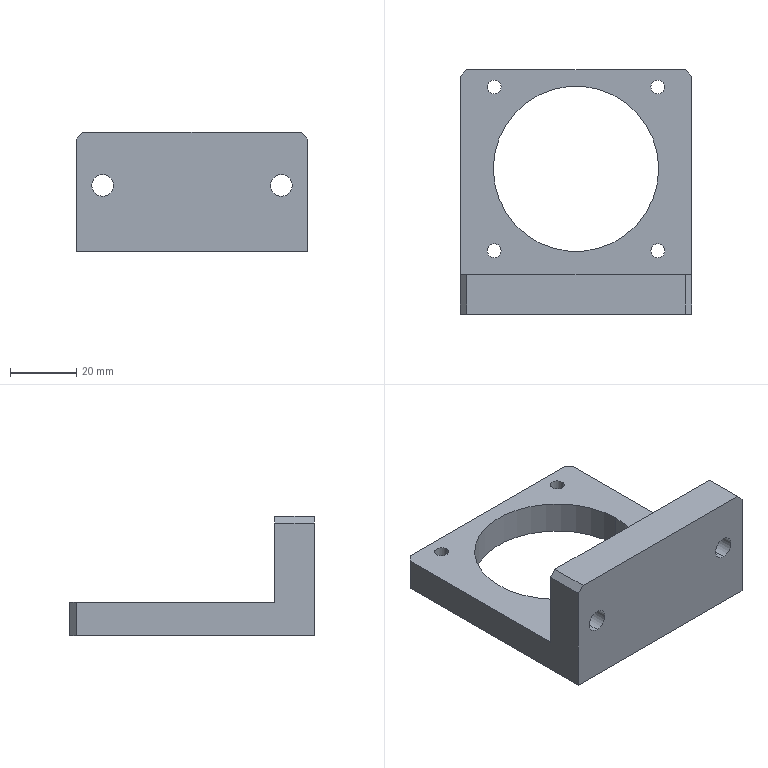Part | NX | features BREP 1 | 1 solid | 32 faces | box 70 x 74 x 36 mm | volume 51715 mm3 | cylinder 18 | plane 14 | commonest cylinder face diameters 4.2 x8 6.6 x4 11 x4 50 x2
STEP:
#1=CARTESIAN_POINT('',(33.,74.,0.));
#2=VERTEX_POINT('',#1);
#3=CARTESIAN_POINT('',(35.,72.,0.));
#4=VERTEX_POINT('',#3);
#5=CARTESIAN_POINT('',(35.,72.,0.));
#6=DIRECTION('',(0.7071,-0.7071,0.));
#7=VECTOR('',#6,1000.);
#8=LINE('',#5,#7);
#9=EDGE_CURVE('',#2,#4,#8,.T.);
#10=ORIENTED_EDGE('',*,*,#9,.F.);
#11=CARTESIAN_POINT('',(33.,74.,10.));
#12=VERTEX_POINT('',#11);
#13=CARTESIAN_POINT('',(33.,74.,0.));
#14=DIRECTION('',(0.,0.,-1.));
#15=VECTOR('',#14,1000.);
#16=LINE('',#13,#15);
#17=EDGE_CURVE('',#12,#2,#16,.T.);
#18=ORIENTED_EDGE('',*,*,#17,.F.);
#19=CARTESIAN_POINT('',(35.,72.,10.));
#20=VERTEX_POINT('',#19);
#21=CARTESIAN_POINT('',(35.,72.,10.));
#22=DIRECTION('',(-0.7071,0.7071,0.));
#23=VECTOR('',#22,1000.);
#24=LINE('',#21,#23);
#25=EDGE_CURVE('',#20,#12,#24,.T.);
#26=ORIENTED_EDGE('',*,*,#25,.F.);
#27=CARTESIAN_POINT('',(35.,72.,10.));
#28=DIRECTION('',(0.,0.,1.));
#29=VECTOR('',#28,1000.);
#30=LINE('',#27,#29);
#31=EDGE_CURVE('',#4,#20,#30,.T.);
#32=ORIENTED_EDGE('',*,*,#31,.F.);
#33=EDGE_LOOP('',(#10,#18,#26,#32));
#34=FACE_BOUND('',#33,.T.);
#35=CARTESIAN_POINT('',(35.,72.,0.));
#36=DIRECTION('',(0.7071,0.7071,0.));
#37=DIRECTION('',(0.,0.,-1.));
#38=AXIS2_PLACEMENT_3D('',#35,#36,#37);
#39=PLANE('',#38);
#40=ADVANCED_FACE('',(#34),#39,.T.);
#41=CARTESIAN_POINT('',(33.,12.,36.));
#42=VERTEX_POINT('',#41);
#43=CARTESIAN_POINT('',(35.,12.,34.));
#44=VERTEX_POINT('',#43);
#45=CARTESIAN_POINT('',(35.,12.,34.));
#46=DIRECTION('',(0.7071,0.,-0.7071));
#47=VECTOR('',#46,1000.);
#48=LINE('',#45,#47);
#49=EDGE_CURVE('',#42,#44,#48,.T.);
#50=ORIENTED_EDGE('',*,*,#49,.F.);
#51=CARTESIAN_POINT('',(33.,0.,36.));
#52=VERTEX_POINT('',#51);
#53=CARTESIAN_POINT('',(33.,12.,36.));
#54=DIRECTION('',(0.,1.,0.));
#55=VECTOR('',#54,1000.);
#56=LINE('',#53,#55);
#57=EDGE_CURVE('',#52,#42,#56,.T.);
#58=ORIENTED_EDGE('',*,*,#57,.F.);
#59=CARTESIAN_POINT('',(35.,0.,34.));
#60=VERTEX_POINT('',#59);
#61=CARTESIAN_POINT('',(35.,0.,34.));
#62=DIRECTION('',(-0.7071,0.,0.7071));
#63=VECTOR('',#62,1000.);
#64=LINE('',#61,#63);
#65=EDGE_CURVE('',#60,#52,#64,.T.);
#66=ORIENTED_EDGE('',*,*,#65,.F.);
#67=CARTESIAN_POINT('',(35.,0.,34.));
#68=DIRECTION('',(0.,-1.,0.));
#69=VECTOR('',#68,1000.);
#70=LINE('',#67,#69);
#71=EDGE_CURVE('',#44,#60,#70,.T.);
#72=ORIENTED_EDGE('',*,*,#71,.F.);
#73=EDGE_LOOP('',(#50,#58,#66,#72));
#74=FACE_BOUND('',#73,.T.);
#75=CARTESIAN_POINT('',(35.,0.,34.));
#76=DIRECTION('',(0.7071,0.,0.7071));
#77=DIRECTION('',(0.,1.,0.));
#78=AXIS2_PLACEMENT_3D('',#75,#76,#77);
#79=PLANE('',#78);
#80=ADVANCED_FACE('',(#74),#79,.T.);
#81=CARTESIAN_POINT('',(-35.,12.,34.));
#82=VERTEX_POINT('',#81);
#83=CARTESIAN_POINT('',(-33.,12.,36.));
#84=VERTEX_POINT('',#83);
#85=CARTESIAN_POINT('',(-33.,12.,36.));
#86=DIRECTION('',(0.7071,0.,0.7071));
#87=VECTOR('',#86,1000.);
#88=LINE('',#85,#87);
#89=EDGE_CURVE('',#82,#84,#88,.T.);
#90=ORIENTED_EDGE('',*,*,#89,.F.);
#91=CARTESIAN_POINT('',(-35.,0.,34.));
#92=VERTEX_POINT('',#91);
#93=CARTESIAN_POINT('',(-35.,0.,34.));
#94=DIRECTION('',(0.,1.,0.));
#95=VECTOR('',#94,1000.);
#96=LINE('',#93,#95);
#97=EDGE_CURVE('',#92,#82,#96,.T.);
#98=ORIENTED_EDGE('',*,*,#97,.F.);
#99=CARTESIAN_POINT('',(-33.,0.,36.));
#100=VERTEX_POINT('',#99);
#101=CARTESIAN_POINT('',(-33.,0.,36.));
#102=DIRECTION('',(-0.7071,0.,-0.7071));
#103=VECTOR('',#102,1000.);
#104=LINE('',#101,#103);
#105=EDGE_CURVE('',#100,#92,#104,.T.);
#106=ORIENTED_EDGE('',*,*,#105,.F.);
#107=CARTESIAN_POINT('',(-33.,0.,36.));
#108=DIRECTION('',(0.,-1.,0.));
#109=VECTOR('',#108,1000.);
#110=LINE('',#107,#109);
#111=EDGE_CURVE('',#84,#100,#110,.T.);
#112=ORIENTED_EDGE('',*,*,#111,.F.);
#113=EDGE_LOOP('',(#90,#98,#106,#112));
#114=FACE_BOUND('',#113,.T.);
#115=CARTESIAN_POINT('',(-33.,0.,36.));
#116=DIRECTION('',(0.7071,0.,-0.7071));
#117=DIRECTION('',(0.,-1.,0.));
#118=AXIS2_PLACEMENT_3D('',#115,#116,#117);
#119=PLANE('',#118);
#120=ADVANCED_FACE('',(#114),#119,.F.);
#121=CARTESIAN_POINT('',(-35.,72.,0.));
#122=VERTEX_POINT('',#121);
#123=CARTESIAN_POINT('',(-33.,74.,0.));
#124=VERTEX_POINT('',#123);
#125=CARTESIAN_POINT('',(-33.,74.,0.));
#126=DIRECTION('',(0.7071,0.7071,0.));
#127=VECTOR('',#126,1000.);
#128=LINE('',#125,#127);
#129=EDGE_CURVE('',#122,#124,#128,.T.);
#130=ORIENTED_EDGE('',*,*,#129,.F.);
#131=CARTESIAN_POINT('',(-35.,72.,10.));
#132=VERTEX_POINT('',#131);
#133=CARTESIAN_POINT('',(-35.,72.,0.));
#134=DIRECTION('',(0.,0.,-1.));
#135=VECTOR('',#134,1000.);
#136=LINE('',#133,#135);
#137=EDGE_CURVE('',#132,#122,#136,.T.);
#138=ORIENTED_EDGE('',*,*,#137,.F.);
#139=CARTESIAN_POINT('',(-33.,74.,10.));
#140=VERTEX_POINT('',#139);
#141=CARTESIAN_POINT('',(-33.,74.,10.));
#142=DIRECTION('',(-0.7071,-0.7071,0.));
#143=VECTOR('',#142,1000.);
#144=LINE('',#141,#143);
#145=EDGE_CURVE('',#140,#132,#144,.T.);
#146=ORIENTED_EDGE('',*,*,#145,.F.);
#147=CARTESIAN_POINT('',(-33.,74.,0.));
#148=DIRECTION('',(0.,0.,1.));
#149=VECTOR('',#148,1000.);
#150=LINE('',#147,#149);
#151=EDGE_CURVE('',#124,#140,#150,.T.);
#152=ORIENTED_EDGE('',*,*,#151,.F.);
#153=EDGE_LOOP('',(#130,#138,#146,#152));
#154=FACE_BOUND('',#153,.T.);
#155=CARTESIAN_POINT('',(-33.,74.,0.));
#156=DIRECTION('',(0.7071,-0.7071,0.));
#157=DIRECTION('',(0.,0.,1.));
#158=AXIS2_PLACEMENT_3D('',#155,#156,#157);
#159=PLANE('',#158);
#160=ADVANCED_FACE('',(#154),#159,.F.);
#161=CARTESIAN_POINT('',(-27.,12.,14.5));
#162=VERTEX_POINT('',#161);
#163=CARTESIAN_POINT('',(-27.,5.2,14.5));
#164=VERTEX_POINT('',#163);
#165=CARTESIAN_POINT('',(-27.,12.,14.5));
#166=DIRECTION('',(0.,1.,0.));
#167=VECTOR('',#166,1000.);
#168=LINE('',#165,#167);
#169=EDGE_CURVE('',#162,#164,#168,.F.);
#170=ORIENTED_EDGE('',*,*,#169,.T.);
#171=CARTESIAN_POINT('',(-27.,5.2,25.5));
#172=VERTEX_POINT('',#171);
#173=CARTESIAN_POINT('',(-27.,5.2,20.));
#174=DIRECTION('',(0.,1.,0.));
#175=DIRECTION('',(0.,0.,1.));
#176=AXIS2_PLACEMENT_3D('',#173,#174,#175);
#177=CIRCLE('',#176,5.5);
#178=EDGE_CURVE('',#172,#164,#177,.T.);
#179=ORIENTED_EDGE('',*,*,#178,.F.);
#180=CARTESIAN_POINT('',(-27.,12.,25.5));
#181=VERTEX_POINT('',#180);
#182=CARTESIAN_POINT('',(-27.,12.,25.5));
#183=DIRECTION('',(0.,1.,0.));
#184=VECTOR('',#183,1000.);
#185=LINE('',#182,#184);
#186=EDGE_CURVE('',#181,#172,#185,.F.);
#187=ORIENTED_EDGE('',*,*,#186,.F.);
#188=CARTESIAN_POINT('',(-27.,12.,20.));
#189=DIRECTION('',(0.,1.,0.));
#190=DIRECTION('',(0.,0.,1.));
#191=AXIS2_PLACEMENT_3D('',#188,#189,#190);
#192=CIRCLE('',#191,5.5);
#193=EDGE_CURVE('',#181,#162,#192,.T.);
#194=ORIENTED_EDGE('',*,*,#193,.T.);
#195=EDGE_LOOP('',(#170,#179,#187,#194));
#196=FACE_BOUND('',#195,.T.);
#197=CARTESIAN_POINT('',(-27.,12.,20.));
#198=DIRECTION('',(0.,1.,0.));
#199=DIRECTION('',(0.,0.,1.));
#200=AXIS2_PLACEMENT_3D('',#197,#198,#199);
#201=CYLINDRICAL_SURFACE('',#200,5.5);
#202=ADVANCED_FACE('',(#196),#201,.F.);
#203=ORIENTED_EDGE('',*,*,#178,.T.);
#204=CARTESIAN_POINT('',(-27.,5.2,20.));
#205=DIRECTION('',(0.,1.,0.));
#206=DIRECTION('',(0.,0.,1.));
#207=AXIS2_PLACEMENT_3D('',#204,#205,#206);
#208=CIRCLE('',#207,5.5);
#209=EDGE_CURVE('',#164,#172,#208,.T.);
#210=ORIENTED_EDGE('',*,*,#209,.T.);
#211=EDGE_LOOP('',(#203,#210));
#212=FACE_BOUND('',#211,.T.);
#213=CARTESIAN_POINT('',(-27.,5.2,23.3));
#214=VERTEX_POINT('',#213);
#215=CARTESIAN_POINT('',(-27.,5.2,16.7));
#216=VERTEX_POINT('',#215);
#217=CARTESIAN_POINT('',(-27.,5.2,20.));
#218=DIRECTION('',(0.,1.,0.));
#219=DIRECTION('',(0.,0.,1.));
#220=AXIS2_PLACEMENT_3D('',#217,#218,#219);
#221=CIRCLE('',#220,3.3);
#222=EDGE_CURVE('',#214,#216,#221,.T.);
#223=ORIENTED_EDGE('',*,*,#222,.F.);
#224=CARTESIAN_POINT('',(-27.,5.2,20.));
#225=DIRECTION('',(0.,1.,0.));
#226=DIRECTION('',(0.,0.,1.));
#227=AXIS2_PLACEMENT_3D('',#224,#225,#226);
#228=CIRCLE('',#227,3.3);
#229=EDGE_CURVE('',#216,#214,#228,.T.);
#230=ORIENTED_EDGE('',*,*,#229,.F.);
#231=EDGE_LOOP('',(#223,#230));
#232=FACE_BOUND('',#231,.T.);
#233=CARTESIAN_POINT('',(-23.7,5.2,20.));
#234=DIRECTION('',(0.,-1.,0.));
#235=DIRECTION('',(0.,0.,-1.));
#236=AXIS2_PLACEMENT_3D('',#233,#234,#235);
#237=PLANE('',#236);
#238=ADVANCED_FACE('',(#212,#232),#237,.F.);
#239=CARTESIAN_POINT('',(-27.,0.,16.7));
#240=VERTEX_POINT('',#239);
#241=CARTESIAN_POINT('',(-27.,12.,16.7));
#242=DIRECTION('',(0.,1.,0.));
#243=VECTOR('',#242,1000.);
#244=LINE('',#241,#243);
#245=EDGE_CURVE('',#216,#240,#244,.F.);
#246=ORIENTED_EDGE('',*,*,#245,.T.);
#247=CARTESIAN_POINT('',(-27.,0.,23.3));
#248=VERTEX_POINT('',#247);
#249=CARTESIAN_POINT('',(-27.,0.,20.));
#250=DIRECTION('',(0.,1.,0.));
#251=DIRECTION('',(0.,0.,1.));
#252=AXIS2_PLACEMENT_3D('',#249,#250,#251);
#253=CIRCLE('',#252,3.3);
#254=EDGE_CURVE('',#248,#240,#253,.T.);
#255=ORIENTED_EDGE('',*,*,#254,.F.);
#256=CARTESIAN_POINT('',(-27.,12.,23.3));
#257=DIRECTION('',(0.,1.,0.));
#258=VECTOR('',#257,1000.);
#259=LINE('',#256,#258);
#260=EDGE_CURVE('',#214,#248,#259,.F.);
#261=ORIENTED_EDGE('',*,*,#260,.F.);
#262=ORIENTED_EDGE('',*,*,#222,.T.);
#263=EDGE_LOOP('',(#246,#255,#261,#262));
#264=FACE_BOUND('',#263,.T.);
#265=CARTESIAN_POINT('',(-27.,12.,20.));
#266=DIRECTION('',(0.,1.,0.));
#267=DIRECTION('',(0.,0.,1.));
#268=AXIS2_PLACEMENT_3D('',#265,#266,#267);
#269=CYLINDRICAL_SURFACE('',#268,3.3);
#270=ADVANCED_FACE('',(#264),#269,.F.);
#271=CARTESIAN_POINT('',(27.,12.,14.5));
#272=VERTEX_POINT('',#271);
#273=CARTESIAN_POINT('',(27.,5.2,14.5));
#274=VERTEX_POINT('',#273);
#275=CARTESIAN_POINT('',(27.,12.,14.5));
#276=DIRECTION('',(0.,1.,0.));
#277=VECTOR('',#276,1000.);
#278=LINE('',#275,#277);
#279=EDGE_CURVE('',#272,#274,#278,.F.);
#280=ORIENTED_EDGE('',*,*,#279,.T.);
#281=CARTESIAN_POINT('',(27.,5.2,25.5));
#282=VERTEX_POINT('',#281);
#283=CARTESIAN_POINT('',(27.,5.2,20.));
#284=DIRECTION('',(0.,1.,0.));
#285=DIRECTION('',(0.,0.,1.));
#286=AXIS2_PLACEMENT_3D('',#283,#284,#285);
#287=CIRCLE('',#286,5.5);
#288=EDGE_CURVE('',#282,#274,#287,.T.);
#289=ORIENTED_EDGE('',*,*,#288,.F.);
#290=CARTESIAN_POINT('',(27.,12.,25.5));
#291=VERTEX_POINT('',#290);
#292=CARTESIAN_POINT('',(27.,12.,25.5));
#293=DIRECTION('',(0.,1.,0.));
#294=VECTOR('',#293,1000.);
#295=LINE('',#292,#294);
#296=EDGE_CURVE('',#291,#282,#295,.F.);
#297=ORIENTED_EDGE('',*,*,#296,.F.);
#298=CARTESIAN_POINT('',(27.,12.,20.));
#299=DIRECTION('',(0.,1.,0.));
#300=DIRECTION('',(0.,0.,1.));
#301=AXIS2_PLACEMENT_3D('',#298,#299,#300);
#302=CIRCLE('',#301,5.5);
#303=EDGE_CURVE('',#291,#272,#302,.T.);
#304=ORIENTED_EDGE('',*,*,#303,.T.);
#305=EDGE_LOOP('',(#280,#289,#297,#304));
#306=FACE_BOUND('',#305,.T.);
#307=CARTESIAN_POINT('',(27.,12.,20.));
#308=DIRECTION('',(0.,1.,0.));
#309=DIRECTION('',(0.,0.,1.));
#310=AXIS2_PLACEMENT_3D('',#307,#308,#309);
#311=CYLINDRICAL_SURFACE('',#310,5.5);
#312=ADVANCED_FACE('',(#306),#311,.F.);
#313=ORIENTED_EDGE('',*,*,#288,.T.);
#314=CARTESIAN_POINT('',(27.,5.2,20.));
#315=DIRECTION('',(0.,1.,0.));
#316=DIRECTION('',(0.,0.,1.));
#317=AXIS2_PLACEMENT_3D('',#314,#315,#316);
#318=CIRCLE('',#317,5.5);
#319=EDGE_CURVE('',#274,#282,#318,.T.);
#320=ORIENTED_EDGE('',*,*,#319,.T.);
#321=EDGE_LOOP('',(#313,#320));
#322=FACE_BOUND('',#321,.T.);
#323=CARTESIAN_POINT('',(27.,5.2,23.3));
#324=VERTEX_POINT('',#323);
#325=CARTESIAN_POINT('',(27.,5.2,16.7));
#326=VERTEX_POINT('',#325);
#327=CARTESIAN_POINT('',(27.,5.2,20.));
#328=DIRECTION('',(0.,1.,0.));
#329=DIRECTION('',(0.,0.,1.));
#330=AXIS2_PLACEMENT_3D('',#327,#328,#329);
#331=CIRCLE('',#330,3.3);
#332=EDGE_CURVE('',#324,#326,#331,.T.);
#333=ORIENTED_EDGE('',*,*,#332,.F.);
#334=CARTESIAN_POINT('',(27.,5.2,20.));
#335=DIRECTION('',(0.,1.,0.));
#336=DIRECTION('',(0.,0.,1.));
#337=AXIS2_PLACEMENT_3D('',#334,#335,#336);
#338=CIRCLE('',#337,3.3);
#339=EDGE_CURVE('',#326,#324,#338,.T.);
#340=ORIENTED_EDGE('',*,*,#339,.F.);
#341=EDGE_LOOP('',(#333,#340));
#342=FACE_BOUND('',#341,.T.);
#343=CARTESIAN_POINT('',(30.3,5.2,20.));
#344=DIRECTION('',(0.,-1.,0.));
#345=DIRECTION('',(0.,0.,-1.));
#346=AXIS2_PLACEMENT_3D('',#343,#344,#345);
#347=PLANE('',#346);
#348=ADVANCED_FACE('',(#322,#342),#347,.F.);
#349=CARTESIAN_POINT('',(27.,0.,16.7));
#350=VERTEX_POINT('',#349);
#351=CARTESIAN_POINT('',(27.,12.,16.7));
#352=DIRECTION('',(0.,1.,0.));
#353=VECTOR('',#352,1000.);
#354=LINE('',#351,#353);
#355=EDGE_CURVE('',#326,#350,#354,.F.);
#356=ORIENTED_EDGE('',*,*,#355,.T.);
#357=CARTESIAN_POINT('',(27.,0.,23.3));
#358=VERTEX_POINT('',#357);
#359=CARTESIAN_POINT('',(27.,0.,20.));
#360=DIRECTION('',(0.,1.,0.));
#361=DIRECTION('',(0.,0.,1.));
#362=AXIS2_PLACEMENT_3D('',#359,#360,#361);
#363=CIRCLE('',#362,3.3);
#364=EDGE_CURVE('',#358,#350,#363,.T.);
#365=ORIENTED_EDGE('',*,*,#364,.F.);
#366=CARTESIAN_POINT('',(27.,12.,23.3));
#367=DIRECTION('',(0.,1.,0.));
#368=VECTOR('',#367,1000.);
#369=LINE('',#366,#368);
#370=EDGE_CURVE('',#324,#358,#369,.F.);
#371=ORIENTED_EDGE('',*,*,#370,.F.);
#372=ORIENTED_EDGE('',*,*,#332,.T.);
#373=EDGE_LOOP('',(#356,#365,#371,#372));
#374=FACE_BOUND('',#373,.T.);
#375=CARTESIAN_POINT('',(27.,12.,20.));
#376=DIRECTION('',(0.,1.,0.));
#377=DIRECTION('',(0.,0.,1.));
#378=AXIS2_PLACEMENT_3D('',#375,#376,#377);
#379=CYLINDRICAL_SURFACE('',#378,3.3);
#380=ADVANCED_FACE('',(#374),#379,.F.);
#381=CARTESIAN_POINT('',(-22.649,68.749,10.));
#382=VERTEX_POINT('',#381);
#383=CARTESIAN_POINT('',(-22.649,68.749,0.));
#384=VERTEX_POINT('',#383);
#385=CARTESIAN_POINT('',(-22.649,68.749,0.));
#386=DIRECTION('',(0.,0.,-1.));
#387=VECTOR('',#386,1000.);
#388=LINE('',#385,#387);
#389=EDGE_CURVE('',#382,#384,#388,.T.);
#390=ORIENTED_EDGE('',*,*,#389,.F.);
#391=CARTESIAN_POINT('',(-26.849,68.749,10.));
#392=VERTEX_POINT('',#391);
#393=CARTESIAN_POINT('',(-24.749,68.749,10.));
#394=DIRECTION('',(0.,0.,-1.));
#395=DIRECTION('',(0.,1.,0.));
#396=AXIS2_PLACEMENT_3D('',#393,#394,#395);
#397=CIRCLE('',#396,2.1);
#398=EDGE_CURVE('',#392,#382,#397,.T.);
#399=ORIENTED_EDGE('',*,*,#398,.F.);
#400=CARTESIAN_POINT('',(-26.849,68.749,0.));
#401=VERTEX_POINT('',#400);
#402=CARTESIAN_POINT('',(-26.849,68.749,0.));
#403=DIRECTION('',(0.,0.,-1.));
#404=VECTOR('',#403,1000.);
#405=LINE('',#402,#404);
#406=EDGE_CURVE('',#392,#401,#405,.T.);
#407=ORIENTED_EDGE('',*,*,#406,.T.);
#408=CARTESIAN_POINT('',(-24.749,68.749,0.));
#409=DIRECTION('',(0.,0.,-1.));
#410=DIRECTION('',(-1.,0.,0.));
#411=AXIS2_PLACEMENT_3D('',#408,#409,#410);
#412=CIRCLE('',#411,2.1);
#413=EDGE_CURVE('',#401,#384,#412,.T.);
#414=ORIENTED_EDGE('',*,*,#413,.T.);
#415=EDGE_LOOP('',(#390,#399,#407,#414));
#416=FACE_BOUND('',#415,.T.);
#417=CARTESIAN_POINT('',(-24.749,68.749,0.));
#418=DIRECTION('',(0.,0.,-1.));
#419=DIRECTION('',(-1.,0.,0.));
#420=AXIS2_PLACEMENT_3D('',#417,#418,#419);
#421=CYLINDRICAL_SURFACE('',#420,2.1);
#422=ADVANCED_FACE('',(#416),#421,.F.);
#423=CARTESIAN_POINT('',(-22.649,19.251,10.));
#424=VERTEX_POINT('',#423);
#425=CARTESIAN_POINT('',(-22.649,19.251,0.));
#426=VERTEX_POINT('',#425);
#427=CARTESIAN_POINT('',(-22.649,19.251,0.));
#428=DIRECTION('',(0.,0.,-1.));
#429=VECTOR('',#428,1000.);
#430=LINE('',#427,#429);
#431=EDGE_CURVE('',#424,#426,#430,.T.);
#432=ORIENTED_EDGE('',*,*,#431,.F.);
#433=CARTESIAN_POINT('',(-26.849,19.251,10.));
#434=VERTEX_POINT('',#433);
#435=CARTESIAN_POINT('',(-24.749,19.251,10.));
#436=DIRECTION('',(0.,0.,-1.));
#437=DIRECTION('',(0.,1.,0.));
#438=AXIS2_PLACEMENT_3D('',#435,#436,#437);
#439=CIRCLE('',#438,2.1);
#440=EDGE_CURVE('',#434,#424,#439,.T.);
#441=ORIENTED_EDGE('',*,*,#440,.F.);
#442=CARTESIAN_POINT('',(-26.849,19.251,0.));
#443=VERTEX_POINT('',#442);
#444=CARTESIAN_POINT('',(-26.849,19.251,0.));
#445=DIRECTION('',(0.,0.,-1.));
#446=VECTOR('',#445,1000.);
#447=LINE('',#444,#446);
#448=EDGE_CURVE('',#434,#443,#447,.T.);
#449=ORIENTED_EDGE('',*,*,#448,.T.);
#450=CARTESIAN_POINT('',(-24.749,19.251,0.));
#451=DIRECTION('',(0.,0.,-1.));
#452=DIRECTION('',(-1.,0.,0.));
#453=AXIS2_PLACEMENT_3D('',#450,#451,#452);
#454=CIRCLE('',#453,2.1);
#455=EDGE_CURVE('',#443,#426,#454,.T.);
#456=ORIENTED_EDGE('',*,*,#455,.T.);
#457=EDGE_LOOP('',(#432,#441,#449,#456));
#458=FACE_BOUND('',#457,.T.);
#459=CARTESIAN_POINT('',(-24.749,19.251,0.));
#460=DIRECTION('',(0.,0.,-1.));
#461=DIRECTION('',(-1.,0.,0.));
#462=AXIS2_PLACEMENT_3D('',#459,#460,#461);
#463=CYLINDRICAL_SURFACE('',#462,2.1);
#464=ADVANCED_FACE('',(#458),#463,.F.);
#465=CARTESIAN_POINT('',(26.849,19.251,10.));
#466=VERTEX_POINT('',#465);
#467=CARTESIAN_POINT('',(26.849,19.251,0.));
#468=VERTEX_POINT('',#467);
#469=CARTESIAN_POINT('',(26.849,19.251,0.));
#470=DIRECTION('',(0.,0.,-1.));
#471=VECTOR('',#470,1000.);
#472=LINE('',#469,#471);
#473=EDGE_CURVE('',#466,#468,#472,.T.);
#474=ORIENTED_EDGE('',*,*,#473,.F.);
#475=CARTESIAN_POINT('',(22.649,19.251,10.));
#476=VERTEX_POINT('',#475);
#477=CARTESIAN_POINT('',(24.749,19.251,10.));
#478=DIRECTION('',(0.,0.,-1.));
#479=DIRECTION('',(0.,1.,0.));
#480=AXIS2_PLACEMENT_3D('',#477,#478,#479);
#481=CIRCLE('',#480,2.1);
#482=EDGE_CURVE('',#476,#466,#481,.T.);
#483=ORIENTED_EDGE('',*,*,#482,.F.);
#484=CARTESIAN_POINT('',(22.649,19.251,0.));
#485=VERTEX_POINT('',#484);
#486=CARTESIAN_POINT('',(22.649,19.251,0.));
#487=DIRECTION('',(0.,0.,-1.));
#488=VECTOR('',#487,1000.);
#489=LINE('',#486,#488);
#490=EDGE_CURVE('',#476,#485,#489,.T.);
#491=ORIENTED_EDGE('',*,*,#490,.T.);
#492=CARTESIAN_POINT('',(24.749,19.251,0.));
#493=DIRECTION('',(0.,0.,-1.));
#494=DIRECTION('',(-1.,0.,0.));
#495=AXIS2_PLACEMENT_3D('',#492,#493,#494);
#496=CIRCLE('',#495,2.1);
#497=EDGE_CURVE('',#485,#468,#496,.T.);
#498=ORIENTED_EDGE('',*,*,#497,.T.);
#499=EDGE_LOOP('',(#474,#483,#491,#498));
#500=FACE_BOUND('',#499,.T.);
#501=CARTESIAN_POINT('',(24.749,19.251,0.));
#502=DIRECTION('',(0.,0.,-1.));
#503=DIRECTION('',(-1.,0.,0.));
#504=AXIS2_PLACEMENT_3D('',#501,#502,#503);
#505=CYLINDRICAL_SURFACE('',#504,2.1);
#506=ADVANCED_FACE('',(#500),#505,.F.);
#507=CARTESIAN_POINT('',(26.849,68.749,10.));
#508=VERTEX_POINT('',#507);
#509=CARTESIAN_POINT('',(26.849,68.749,0.));
#510=VERTEX_POINT('',#509);
#511=CARTESIAN_POINT('',(26.849,68.749,0.));
#512=DIRECTION('',(0.,0.,-1.));
#513=VECTOR('',#512,1000.);
#514=LINE('',#511,#513);
#515=EDGE_CURVE('',#508,#510,#514,.T.);
#516=ORIENTED_EDGE('',*,*,#515,.F.);
#517=CARTESIAN_POINT('',(22.649,68.749,10.));
#518=VERTEX_POINT('',#517);
#519=CARTESIAN_POINT('',(24.749,68.749,10.));
#520=DIRECTION('',(0.,0.,-1.));
#521=DIRECTION('',(0.,1.,0.));
#522=AXIS2_PLACEMENT_3D('',#519,#520,#521);
#523=CIRCLE('',#522,2.1);
#524=EDGE_CURVE('',#518,#508,#523,.T.);
#525=ORIENTED_EDGE('',*,*,#524,.F.);
#526=CARTESIAN_POINT('',(22.649,68.749,0.));
#527=VERTEX_POINT('',#526);
#528=CARTESIAN_POINT('',(22.649,68.749,0.));
#529=DIRECTION('',(0.,0.,-1.));
#530=VECTOR('',#529,1000.);
#531=LINE('',#528,#530);
#532=EDGE_CURVE('',#518,#527,#531,.T.);
#533=ORIENTED_EDGE('',*,*,#532,.T.);
#534=CARTESIAN_POINT('',(24.749,68.749,0.));
#535=DIRECTION('',(0.,0.,-1.));
#536=DIRECTION('',(-1.,0.,0.));
#537=AXIS2_PLACEMENT_3D('',#534,#535,#536);
#538=CIRCLE('',#537,2.1);
#539=EDGE_CURVE('',#527,#510,#538,.T.);
#540=ORIENTED_EDGE('',*,*,#539,.T.);
#541=EDGE_LOOP('',(#516,#525,#533,#540));
#542=FACE_BOUND('',#541,.T.);
#543=CARTESIAN_POINT('',(24.749,68.749,0.));
#544=DIRECTION('',(0.,0.,-1.));
#545=DIRECTION('',(-1.,0.,0.));
#546=AXIS2_PLACEMENT_3D('',#543,#544,#545);
#547=CYLINDRICAL_SURFACE('',#546,2.1);
#548=ADVANCED_FACE('',(#542),#547,.F.);
#549=CARTESIAN_POINT('',(25.,44.,10.));
#550=VERTEX_POINT('',#549);
#551=CARTESIAN_POINT('',(25.,44.,0.));
#552=VERTEX_POINT('',#551);
#553=CARTESIAN_POINT('',(25.,44.,36.));
#554=DIRECTION('',(0.,0.,-1.));
#555=VECTOR('',#554,1000.);
#556=LINE('',#553,#555);
#557=EDGE_CURVE('',#550,#552,#556,.T.);
#558=ORIENTED_EDGE('',*,*,#557,.F.);
#559=CARTESIAN_POINT('',(-25.,44.,10.));
#560=VERTEX_POINT('',#559);
#561=CARTESIAN_POINT('',(0.,44.,10.));
#562=DIRECTION('',(0.,0.,-1.));
#563=DIRECTION('',(0.,1.,0.));
#564=AXIS2_PLACEMENT_3D('',#561,#562,#563);
#565=CIRCLE('',#564,25.);
#566=EDGE_CURVE('',#560,#550,#565,.T.);
#567=ORIENTED_EDGE('',*,*,#566,.F.);
#568=CARTESIAN_POINT('',(-25.,44.,0.));
#569=VERTEX_POINT('',#568);
#570=CARTESIAN_POINT('',(-25.,44.,36.));
#571=DIRECTION('',(0.,0.,-1.));
#572=VECTOR('',#571,1000.);
#573=LINE('',#570,#572);
#574=EDGE_CURVE('',#560,#569,#573,.T.);
#575=ORIENTED_EDGE('',*,*,#574,.T.);
#576=CARTESIAN_POINT('',(0.,44.,0.));
#577=DIRECTION('',(0.,0.,-1.));
#578=DIRECTION('',(-1.,0.,0.));
#579=AXIS2_PLACEMENT_3D('',#576,#577,#578);
#580=CIRCLE('',#579,25.);
#581=EDGE_CURVE('',#569,#552,#580,.T.);
#582=ORIENTED_EDGE('',*,*,#581,.T.);
#583=EDGE_LOOP('',(#558,#567,#575,#582));
#584=FACE_BOUND('',#583,.T.);
#585=CARTESIAN_POINT('',(0.,44.,36.));
#586=DIRECTION('',(0.,0.,-1.));
#587=DIRECTION('',(-1.,0.,0.));
#588=AXIS2_PLACEMENT_3D('',#585,#586,#587);
#589=CYLINDRICAL_SURFACE('',#588,25.);
#590=ADVANCED_FACE('',(#584),#589,.F.);
#591=CARTESIAN_POINT('',(-35.,12.,10.));
#592=VERTEX_POINT('',#591);
#593=CARTESIAN_POINT('',(-35.,74.,10.));
#594=DIRECTION('',(0.,-1.,0.));
#595=VECTOR('',#594,1000.);
#596=LINE('',#593,#595);
#597=EDGE_CURVE('',#132,#592,#596,.T.);
#598=ORIENTED_EDGE('',*,*,#597,.F.);
#599=ORIENTED_EDGE('',*,*,#137,.T.);
#600=CARTESIAN_POINT('',(-35.,0.,0.));
#601=VERTEX_POINT('',#600);
#602=CARTESIAN_POINT('',(-35.,0.,0.));
#603=DIRECTION('',(0.,1.,0.));
#604=VECTOR('',#603,1000.);
#605=LINE('',#602,#604);
#606=EDGE_CURVE('',#601,#122,#605,.T.);
#607=ORIENTED_EDGE('',*,*,#606,.F.);
#608=CARTESIAN_POINT('',(-35.,0.,0.));
#609=DIRECTION('',(0.,0.,-1.));
#610=VECTOR('',#609,1000.);
#611=LINE('',#608,#610);
#612=EDGE_CURVE('',#92,#601,#611,.T.);
#613=ORIENTED_EDGE('',*,*,#612,.F.);
#614=ORIENTED_EDGE('',*,*,#97,.T.);
#615=CARTESIAN_POINT('',(-35.,12.,36.));
#616=DIRECTION('',(0.,0.,1.));
#617=VECTOR('',#616,1000.);
#618=LINE('',#615,#617);
#619=EDGE_CURVE('',#592,#82,#618,.T.);
#620=ORIENTED_EDGE('',*,*,#619,.F.);
#621=EDGE_LOOP('',(#598,#599,#607,#613,#614,#620));
#622=FACE_BOUND('',#621,.T.);
#623=CARTESIAN_POINT('',(-35.,0.,0.));
#624=DIRECTION('',(1.,0.,0.));
#625=DIRECTION('',(0.,0.,-1.));
#626=AXIS2_PLACEMENT_3D('',#623,#624,#625);
#627=PLANE('',#626);
#628=ADVANCED_FACE('',(#622),#627,.F.);
#629=CARTESIAN_POINT('',(35.,12.,10.));
#630=VERTEX_POINT('',#629);
#631=CARTESIAN_POINT('',(35.,12.,36.));
#632=DIRECTION('',(0.,0.,1.));
#633=VECTOR('',#632,1000.);
#634=LINE('',#631,#633);
#635=EDGE_CURVE('',#630,#44,#634,.T.);
#636=ORIENTED_EDGE('',*,*,#635,.T.);
#637=ORIENTED_EDGE('',*,*,#71,.T.);
#638=CARTESIAN_POINT('',(35.,0.,0.));
#639=VERTEX_POINT('',#638);
#640=CARTESIAN_POINT('',(35.,0.,0.));
#641=DIRECTION('',(0.,0.,-1.));
#642=VECTOR('',#641,1000.);
#643=LINE('',#640,#642);
#644=EDGE_CURVE('',#60,#639,#643,.T.);
#645=ORIENTED_EDGE('',*,*,#644,.T.);
#646=CARTESIAN_POINT('',(35.,0.,0.));
#647=DIRECTION('',(0.,1.,0.));
#648=VECTOR('',#647,1000.);
#649=LINE('',#646,#648);
#650=EDGE_CURVE('',#639,#4,#649,.T.);
#651=ORIENTED_EDGE('',*,*,#650,.T.);
#652=ORIENTED_EDGE('',*,*,#31,.T.);
#653=CARTESIAN_POINT('',(35.,74.,10.));
#654=DIRECTION('',(0.,-1.,0.));
#655=VECTOR('',#654,1000.);
#656=LINE('',#653,#655);
#657=EDGE_CURVE('',#20,#630,#656,.T.);
#658=ORIENTED_EDGE('',*,*,#657,.T.);
#659=EDGE_LOOP('',(#636,#637,#645,#651,#652,#658));
#660=FACE_BOUND('',#659,.T.);
#661=CARTESIAN_POINT('',(35.,0.,0.));
#662=DIRECTION('',(1.,0.,0.));
#663=DIRECTION('',(0.,0.,-1.));
#664=AXIS2_PLACEMENT_3D('',#661,#662,#663);
#665=PLANE('',#664);
#666=ADVANCED_FACE('',(#660),#665,.T.);
#667=CARTESIAN_POINT('',(35.,0.,36.));
#668=DIRECTION('',(-1.,0.,0.));
#669=VECTOR('',#668,1000.);
#670=LINE('',#667,#669);
#671=EDGE_CURVE('',#52,#100,#670,.T.);
#672=ORIENTED_EDGE('',*,*,#671,.T.);
#673=ORIENTED_EDGE('',*,*,#105,.T.);
#674=ORIENTED_EDGE('',*,*,#612,.T.);
#675=CARTESIAN_POINT('',(35.,0.,0.));
#676=DIRECTION('',(-1.,0.,0.));
#677=VECTOR('',#676,1000.);
#678=LINE('',#675,#677);
#679=EDGE_CURVE('',#639,#601,#678,.T.);
#680=ORIENTED_EDGE('',*,*,#679,.F.);
#681=ORIENTED_EDGE('',*,*,#644,.F.);
#682=ORIENTED_EDGE('',*,*,#65,.T.);
#683=EDGE_LOOP('',(#672,#673,#674,#680,#681,#682));
#684=FACE_BOUND('',#683,.T.);
#685=ORIENTED_EDGE('',*,*,#364,.T.);
#686=CARTESIAN_POINT('',(27.,0.,20.));
#687=DIRECTION('',(0.,1.,0.));
#688=DIRECTION('',(0.,0.,1.));
#689=AXIS2_PLACEMENT_3D('',#686,#687,#688);
#690=CIRCLE('',#689,3.3);
#691=EDGE_CURVE('',#350,#358,#690,.T.);
#692=ORIENTED_EDGE('',*,*,#691,.T.);
#693=EDGE_LOOP('',(#685,#692));
#694=FACE_BOUND('',#693,.T.);
#695=ORIENTED_EDGE('',*,*,#254,.T.);
#696=CARTESIAN_POINT('',(-27.,0.,20.));
#697=DIRECTION('',(0.,1.,0.));
#698=DIRECTION('',(0.,0.,1.));
#699=AXIS2_PLACEMENT_3D('',#696,#697,#698);
#700=CIRCLE('',#699,3.3);
#701=EDGE_CURVE('',#240,#248,#700,.T.);
#702=ORIENTED_EDGE('',*,*,#701,.T.);
#703=EDGE_LOOP('',(#695,#702));
#704=FACE_BOUND('',#703,.T.);
#705=CARTESIAN_POINT('',(35.,0.,0.));
#706=DIRECTION('',(0.,1.,0.));
#707=DIRECTION('',(0.,0.,1.));
#708=AXIS2_PLACEMENT_3D('',#705,#706,#707);
#709=PLANE('',#708);
#710=ADVANCED_FACE('',(#684,#694,#704),#709,.F.);
#711=CARTESIAN_POINT('',(35.,12.,36.));
#712=DIRECTION('',(-1.,0.,0.));
#713=VECTOR('',#712,1000.);
#714=LINE('',#711,#713);
#715=EDGE_CURVE('',#42,#84,#714,.T.);
#716=ORIENTED_EDGE('',*,*,#715,.T.);
#717=ORIENTED_EDGE('',*,*,#111,.T.);
#718=ORIENTED_EDGE('',*,*,#671,.F.);
#719=ORIENTED_EDGE('',*,*,#57,.T.);
#720=EDGE_LOOP('',(#716,#717,#718,#719));
#721=FACE_BOUND('',#720,.T.);
#722=CARTESIAN_POINT('',(35.,0.,36.));
#723=DIRECTION('',(0.,0.,-1.));
#724=DIRECTION('',(0.,1.,0.));
#725=AXIS2_PLACEMENT_3D('',#722,#723,#724);
#726=PLANE('',#725);
#727=ADVANCED_FACE('',(#721),#726,.F.);
#728=ORIENTED_EDGE('',*,*,#619,.T.);
#729=ORIENTED_EDGE('',*,*,#89,.T.);
#730=ORIENTED_EDGE('',*,*,#715,.F.);
#731=ORIENTED_EDGE('',*,*,#49,.T.);
#732=ORIENTED_EDGE('',*,*,#635,.F.);
#733=CARTESIAN_POINT('',(35.,12.,10.));
#734=DIRECTION('',(-1.,0.,0.));
#735=VECTOR('',#734,1000.);
#736=LINE('',#733,#735);
#737=EDGE_CURVE('',#630,#592,#736,.T.);
#738=ORIENTED_EDGE('',*,*,#737,.T.);
#739=EDGE_LOOP('',(#728,#729,#730,#731,#732,#738));
#740=FACE_BOUND('',#739,.T.);
#741=ORIENTED_EDGE('',*,*,#303,.F.);
#742=CARTESIAN_POINT('',(27.,12.,20.));
#743=DIRECTION('',(0.,1.,0.));
#744=DIRECTION('',(0.,0.,1.));
#745=AXIS2_PLACEMENT_3D('',#742,#743,#744);
#746=CIRCLE('',#745,5.5);
#747=EDGE_CURVE('',#272,#291,#746,.T.);
#748=ORIENTED_EDGE('',*,*,#747,.F.);
#749=EDGE_LOOP('',(#741,#748));
#750=FACE_BOUND('',#749,.T.);
#751=ORIENTED_EDGE('',*,*,#193,.F.);
#752=CARTESIAN_POINT('',(-27.,12.,20.));
#753=DIRECTION('',(0.,1.,0.));
#754=DIRECTION('',(0.,0.,1.));
#755=AXIS2_PLACEMENT_3D('',#752,#753,#754);
#756=CIRCLE('',#755,5.5);
#757=EDGE_CURVE('',#162,#181,#756,.T.);
#758=ORIENTED_EDGE('',*,*,#757,.F.);
#759=EDGE_LOOP('',(#751,#758));
#760=FACE_BOUND('',#759,.T.);
#761=CARTESIAN_POINT('',(35.,12.,36.));
#762=DIRECTION('',(0.,-1.,0.));
#763=DIRECTION('',(0.,0.,-1.));
#764=AXIS2_PLACEMENT_3D('',#761,#762,#763);
#765=PLANE('',#764);
#766=ADVANCED_FACE('',(#740,#750,#760),#765,.F.);
#767=CARTESIAN_POINT('',(35.,74.,10.));
#768=DIRECTION('',(-1.,0.,0.));
#769=VECTOR('',#768,1000.);
#770=LINE('',#767,#769);
#771=EDGE_CURVE('',#12,#140,#770,.T.);
#772=ORIENTED_EDGE('',*,*,#771,.T.);
#773=ORIENTED_EDGE('',*,*,#145,.T.);
#774=ORIENTED_EDGE('',*,*,#597,.T.);
#775=ORIENTED_EDGE('',*,*,#737,.F.);
#776=ORIENTED_EDGE('',*,*,#657,.F.);
#777=ORIENTED_EDGE('',*,*,#25,.T.);
#778=EDGE_LOOP('',(#772,#773,#774,#775,#776,#777));
#779=FACE_BOUND('',#778,.T.);
#780=ORIENTED_EDGE('',*,*,#566,.T.);
#781=CARTESIAN_POINT('',(0.,44.,10.));
#782=DIRECTION('',(0.,0.,-1.));
#783=DIRECTION('',(0.,1.,0.));
#784=AXIS2_PLACEMENT_3D('',#781,#782,#783);
#785=CIRCLE('',#784,25.);
#786=EDGE_CURVE('',#550,#560,#785,.T.);
#787=ORIENTED_EDGE('',*,*,#786,.T.);
#788=EDGE_LOOP('',(#780,#787));
#789=FACE_BOUND('',#788,.T.);
#790=ORIENTED_EDGE('',*,*,#524,.T.);
#791=CARTESIAN_POINT('',(24.749,68.749,10.));
#792=DIRECTION('',(0.,0.,-1.));
#793=DIRECTION('',(0.,1.,0.));
#794=AXIS2_PLACEMENT_3D('',#791,#792,#793);
#795=CIRCLE('',#794,2.1);
#796=EDGE_CURVE('',#508,#518,#795,.T.);
#797=ORIENTED_EDGE('',*,*,#796,.T.);
#798=EDGE_LOOP('',(#790,#797));
#799=FACE_BOUND('',#798,.T.);
#800=ORIENTED_EDGE('',*,*,#482,.T.);
#801=CARTESIAN_POINT('',(24.749,19.251,10.));
#802=DIRECTION('',(0.,0.,-1.));
#803=DIRECTION('',(0.,1.,0.));
#804=AXIS2_PLACEMENT_3D('',#801,#802,#803);
#805=CIRCLE('',#804,2.1);
#806=EDGE_CURVE('',#466,#476,#805,.T.);
#807=ORIENTED_EDGE('',*,*,#806,.T.);
#808=EDGE_LOOP('',(#800,#807));
#809=FACE_BOUND('',#808,.T.);
#810=ORIENTED_EDGE('',*,*,#440,.T.);
#811=CARTESIAN_POINT('',(-24.749,19.251,10.));
#812=DIRECTION('',(0.,0.,-1.));
#813=DIRECTION('',(0.,1.,0.));
#814=AXIS2_PLACEMENT_3D('',#811,#812,#813);
#815=CIRCLE('',#814,2.1);
#816=EDGE_CURVE('',#424,#434,#815,.T.);
#817=ORIENTED_EDGE('',*,*,#816,.T.);
#818=EDGE_LOOP('',(#810,#817));
#819=FACE_BOUND('',#818,.T.);
#820=ORIENTED_EDGE('',*,*,#398,.T.);
#821=CARTESIAN_POINT('',(-24.749,68.749,10.));
#822=DIRECTION('',(0.,0.,-1.));
#823=DIRECTION('',(0.,1.,0.));
#824=AXIS2_PLACEMENT_3D('',#821,#822,#823);
#825=CIRCLE('',#824,2.1);
#826=EDGE_CURVE('',#382,#392,#825,.T.);
#827=ORIENTED_EDGE('',*,*,#826,.T.);
#828=EDGE_LOOP('',(#820,#827));
#829=FACE_BOUND('',#828,.T.);
#830=CARTESIAN_POINT('',(35.,74.,10.));
#831=DIRECTION('',(0.,0.,-1.));
#832=DIRECTION('',(0.,1.,0.));
#833=AXIS2_PLACEMENT_3D('',#830,#831,#832);
#834=PLANE('',#833);
#835=ADVANCED_FACE('',(#779,#789,#799,#809,#819,#829),#834,.F.);
#836=CARTESIAN_POINT('',(35.,74.,0.));
#837=DIRECTION('',(-1.,0.,0.));
#838=VECTOR('',#837,1000.);
#839=LINE('',#836,#838);
#840=EDGE_CURVE('',#2,#124,#839,.T.);
#841=ORIENTED_EDGE('',*,*,#840,.T.);
#842=ORIENTED_EDGE('',*,*,#151,.T.);
#843=ORIENTED_EDGE('',*,*,#771,.F.);
#844=ORIENTED_EDGE('',*,*,#17,.T.);
#845=EDGE_LOOP('',(#841,#842,#843,#844));
#846=FACE_BOUND('',#845,.T.);
#847=CARTESIAN_POINT('',(35.,74.,0.));
#848=DIRECTION('',(0.,-1.,0.));
#849=DIRECTION('',(0.,0.,-1.));
#850=AXIS2_PLACEMENT_3D('',#847,#848,#849);
#851=PLANE('',#850);
#852=ADVANCED_FACE('',(#846),#851,.F.);
#853=ORIENTED_EDGE('',*,*,#606,.T.);
#854=ORIENTED_EDGE('',*,*,#129,.T.);
#855=ORIENTED_EDGE('',*,*,#840,.F.);
#856=ORIENTED_EDGE('',*,*,#9,.T.);
#857=ORIENTED_EDGE('',*,*,#650,.F.);
#858=ORIENTED_EDGE('',*,*,#679,.T.);
#859=EDGE_LOOP('',(#853,#854,#855,#856,#857,#858));
#860=FACE_BOUND('',#859,.T.);
#861=ORIENTED_EDGE('',*,*,#581,.F.);
#862=CARTESIAN_POINT('',(0.,44.,0.));
#863=DIRECTION('',(0.,0.,-1.));
#864=DIRECTION('',(-1.,0.,0.));
#865=AXIS2_PLACEMENT_3D('',#862,#863,#864);
#866=CIRCLE('',#865,25.);
#867=EDGE_CURVE('',#552,#569,#866,.T.);
#868=ORIENTED_EDGE('',*,*,#867,.F.);
#869=EDGE_LOOP('',(#861,#868));
#870=FACE_BOUND('',#869,.T.);
#871=ORIENTED_EDGE('',*,*,#539,.F.);
#872=CARTESIAN_POINT('',(24.749,68.749,0.));
#873=DIRECTION('',(0.,0.,-1.));
#874=DIRECTION('',(-1.,0.,0.));
#875=AXIS2_PLACEMENT_3D('',#872,#873,#874);
#876=CIRCLE('',#875,2.1);
#877=EDGE_CURVE('',#510,#527,#876,.T.);
#878=ORIENTED_EDGE('',*,*,#877,.F.);
#879=EDGE_LOOP('',(#871,#878));
#880=FACE_BOUND('',#879,.T.);
#881=ORIENTED_EDGE('',*,*,#497,.F.);
#882=CARTESIAN_POINT('',(24.749,19.251,0.));
#883=DIRECTION('',(0.,0.,-1.));
#884=DIRECTION('',(-1.,0.,0.));
#885=AXIS2_PLACEMENT_3D('',#882,#883,#884);
#886=CIRCLE('',#885,2.1);
#887=EDGE_CURVE('',#468,#485,#886,.T.);
#888=ORIENTED_EDGE('',*,*,#887,.F.);
#889=EDGE_LOOP('',(#881,#888));
#890=FACE_BOUND('',#889,.T.);
#891=ORIENTED_EDGE('',*,*,#455,.F.);
#892=CARTESIAN_POINT('',(-24.749,19.251,0.));
#893=DIRECTION('',(0.,0.,-1.));
#894=DIRECTION('',(-1.,0.,0.));
#895=AXIS2_PLACEMENT_3D('',#892,#893,#894);
#896=CIRCLE('',#895,2.1);
#897=EDGE_CURVE('',#426,#443,#896,.T.);
#898=ORIENTED_EDGE('',*,*,#897,.F.);
#899=EDGE_LOOP('',(#891,#898));
#900=FACE_BOUND('',#899,.T.);
#901=ORIENTED_EDGE('',*,*,#413,.F.);
#902=CARTESIAN_POINT('',(-24.749,68.749,0.));
#903=DIRECTION('',(0.,0.,-1.));
#904=DIRECTION('',(-1.,0.,0.));
#905=AXIS2_PLACEMENT_3D('',#902,#903,#904);
#906=CIRCLE('',#905,2.1);
#907=EDGE_CURVE('',#384,#401,#906,.T.);
#908=ORIENTED_EDGE('',*,*,#907,.F.);
#909=EDGE_LOOP('',(#901,#908));
#910=FACE_BOUND('',#909,.T.);
#911=CARTESIAN_POINT('',(35.,0.,0.));
#912=DIRECTION('',(0.,0.,1.));
#913=DIRECTION('',(1.,0.,0.));
#914=AXIS2_PLACEMENT_3D('',#911,#912,#913);
#915=PLANE('',#914);
#916=ADVANCED_FACE('',(#860,#870,#880,#890,#900,#910),#915,.F.);
#917=ORIENTED_EDGE('',*,*,#786,.F.);
#918=ORIENTED_EDGE('',*,*,#557,.T.);
#919=ORIENTED_EDGE('',*,*,#867,.T.);
#920=ORIENTED_EDGE('',*,*,#574,.F.);
#921=EDGE_LOOP('',(#917,#918,#919,#920));
#922=FACE_BOUND('',#921,.T.);
#923=CARTESIAN_POINT('',(0.,44.,36.));
#924=DIRECTION('',(0.,0.,-1.));
#925=DIRECTION('',(-1.,0.,0.));
#926=AXIS2_PLACEMENT_3D('',#923,#924,#925);
#927=CYLINDRICAL_SURFACE('',#926,25.);
#928=ADVANCED_FACE('',(#922),#927,.F.);
#929=ORIENTED_EDGE('',*,*,#796,.F.);
#930=ORIENTED_EDGE('',*,*,#515,.T.);
#931=ORIENTED_EDGE('',*,*,#877,.T.);
#932=ORIENTED_EDGE('',*,*,#532,.F.);
#933=EDGE_LOOP('',(#929,#930,#931,#932));
#934=FACE_BOUND('',#933,.T.);
#935=CARTESIAN_POINT('',(24.749,68.749,0.));
#936=DIRECTION('',(0.,0.,-1.));
#937=DIRECTION('',(-1.,0.,0.));
#938=AXIS2_PLACEMENT_3D('',#935,#936,#937);
#939=CYLINDRICAL_SURFACE('',#938,2.1);
#940=ADVANCED_FACE('',(#934),#939,.F.);
#941=ORIENTED_EDGE('',*,*,#806,.F.);
#942=ORIENTED_EDGE('',*,*,#473,.T.);
#943=ORIENTED_EDGE('',*,*,#887,.T.);
#944=ORIENTED_EDGE('',*,*,#490,.F.);
#945=EDGE_LOOP('',(#941,#942,#943,#944));
#946=FACE_BOUND('',#945,.T.);
#947=CARTESIAN_POINT('',(24.749,19.251,0.));
#948=DIRECTION('',(0.,0.,-1.));
#949=DIRECTION('',(-1.,0.,0.));
#950=AXIS2_PLACEMENT_3D('',#947,#948,#949);
#951=CYLINDRICAL_SURFACE('',#950,2.1);
#952=ADVANCED_FACE('',(#946),#951,.F.);
#953=ORIENTED_EDGE('',*,*,#816,.F.);
#954=ORIENTED_EDGE('',*,*,#431,.T.);
#955=ORIENTED_EDGE('',*,*,#897,.T.);
#956=ORIENTED_EDGE('',*,*,#448,.F.);
#957=EDGE_LOOP('',(#953,#954,#955,#956));
#958=FACE_BOUND('',#957,.T.);
#959=CARTESIAN_POINT('',(-24.749,19.251,0.));
#960=DIRECTION('',(0.,0.,-1.));
#961=DIRECTION('',(-1.,0.,0.));
#962=AXIS2_PLACEMENT_3D('',#959,#960,#961);
#963=CYLINDRICAL_SURFACE('',#962,2.1);
#964=ADVANCED_FACE('',(#958),#963,.F.);
#965=ORIENTED_EDGE('',*,*,#826,.F.);
#966=ORIENTED_EDGE('',*,*,#389,.T.);
#967=ORIENTED_EDGE('',*,*,#907,.T.);
#968=ORIENTED_EDGE('',*,*,#406,.F.);
#969=EDGE_LOOP('',(#965,#966,#967,#968));
#970=FACE_BOUND('',#969,.T.);
#971=CARTESIAN_POINT('',(-24.749,68.749,0.));
#972=DIRECTION('',(0.,0.,-1.));
#973=DIRECTION('',(-1.,0.,0.));
#974=AXIS2_PLACEMENT_3D('',#971,#972,#973);
#975=CYLINDRICAL_SURFACE('',#974,2.1);
#976=ADVANCED_FACE('',(#970),#975,.F.);
#977=ORIENTED_EDGE('',*,*,#691,.F.);
#978=ORIENTED_EDGE('',*,*,#355,.F.);
#979=ORIENTED_EDGE('',*,*,#339,.T.);
#980=ORIENTED_EDGE('',*,*,#370,.T.);
#981=EDGE_LOOP('',(#977,#978,#979,#980));
#982=FACE_BOUND('',#981,.T.);
#983=CARTESIAN_POINT('',(27.,12.,20.));
#984=DIRECTION('',(0.,1.,0.));
#985=DIRECTION('',(0.,0.,1.));
#986=AXIS2_PLACEMENT_3D('',#983,#984,#985);
#987=CYLINDRICAL_SURFACE('',#986,3.3);
#988=ADVANCED_FACE('',(#982),#987,.F.);
#989=ORIENTED_EDGE('',*,*,#319,.F.);
#990=ORIENTED_EDGE('',*,*,#279,.F.);
#991=ORIENTED_EDGE('',*,*,#747,.T.);
#992=ORIENTED_EDGE('',*,*,#296,.T.);
#993=EDGE_LOOP('',(#989,#990,#991,#992));
#994=FACE_BOUND('',#993,.T.);
#995=CARTESIAN_POINT('',(27.,12.,20.));
#996=DIRECTION('',(0.,1.,0.));
#997=DIRECTION('',(0.,0.,1.));
#998=AXIS2_PLACEMENT_3D('',#995,#996,#997);
#999=CYLINDRICAL_SURFACE('',#998,5.5);
#1000=ADVANCED_FACE('',(#994),#999,.F.);
#1001=ORIENTED_EDGE('',*,*,#701,.F.);
#1002=ORIENTED_EDGE('',*,*,#245,.F.);
#1003=ORIENTED_EDGE('',*,*,#229,.T.);
#1004=ORIENTED_EDGE('',*,*,#260,.T.);
#1005=EDGE_LOOP('',(#1001,#1002,#1003,#1004));
#1006=FACE_BOUND('',#1005,.T.);
#1007=CARTESIAN_POINT('',(-27.,12.,20.));
#1008=DIRECTION('',(0.,1.,0.));
#1009=DIRECTION('',(0.,0.,1.));
#1010=AXIS2_PLACEMENT_3D('',#1007,#1008,#1009);
#1011=CYLINDRICAL_SURFACE('',#1010,3.3);
#1012=ADVANCED_FACE('',(#1006),#1011,.F.);
#1013=ORIENTED_EDGE('',*,*,#209,.F.);
#1014=ORIENTED_EDGE('',*,*,#169,.F.);
#1015=ORIENTED_EDGE('',*,*,#757,.T.);
#1016=ORIENTED_EDGE('',*,*,#186,.T.);
#1017=EDGE_LOOP('',(#1013,#1014,#1015,#1016));
#1018=FACE_BOUND('',#1017,.T.);
#1019=CARTESIAN_POINT('',(-27.,12.,20.));
#1020=DIRECTION('',(0.,1.,0.));
#1021=DIRECTION('',(0.,0.,1.));
#1022=AXIS2_PLACEMENT_3D('',#1019,#1020,#1021);
#1023=CYLINDRICAL_SURFACE('',#1022,5.5);
#1024=ADVANCED_FACE('',(#1018),#1023,.F.);
#1025=CLOSED_SHELL('',(#40,#80,#120,#160,#202,#238,#270,#312,#348,#380,#422,#464,#506,#548,#590,#628,#666,#710,#727,#766,#835,#852,#916,#928,#940,#952,#964,#976,#988,#1000,#1012,#1024));
#1026=MANIFOLD_SOLID_BREP('',#1025);
#1027=(LENGTH_UNIT()NAMED_UNIT(*)SI_UNIT(.MILLI.,.METRE.));
#1028=UNCERTAINTY_MEASURE_WITH_UNIT(LENGTH_MEASURE(0.00001),#1027,'','');
#1029=(NAMED_UNIT(*)PLANE_ANGLE_UNIT()SI_UNIT($,.RADIAN.));
#1030=(NAMED_UNIT(*)SI_UNIT($,.STERADIAN.)SOLID_ANGLE_UNIT());
#1031=(GEOMETRIC_REPRESENTATION_CONTEXT(3)GLOBAL_UNCERTAINTY_ASSIGNED_CONTEXT((#1028))GLOBAL_UNIT_ASSIGNED_CONTEXT((#1027,#1029,#1030))REPRESENTATION_CONTEXT('',''));
#1032=ADVANCED_BREP_SHAPE_REPRESENTATION('',(#1026),#1031);